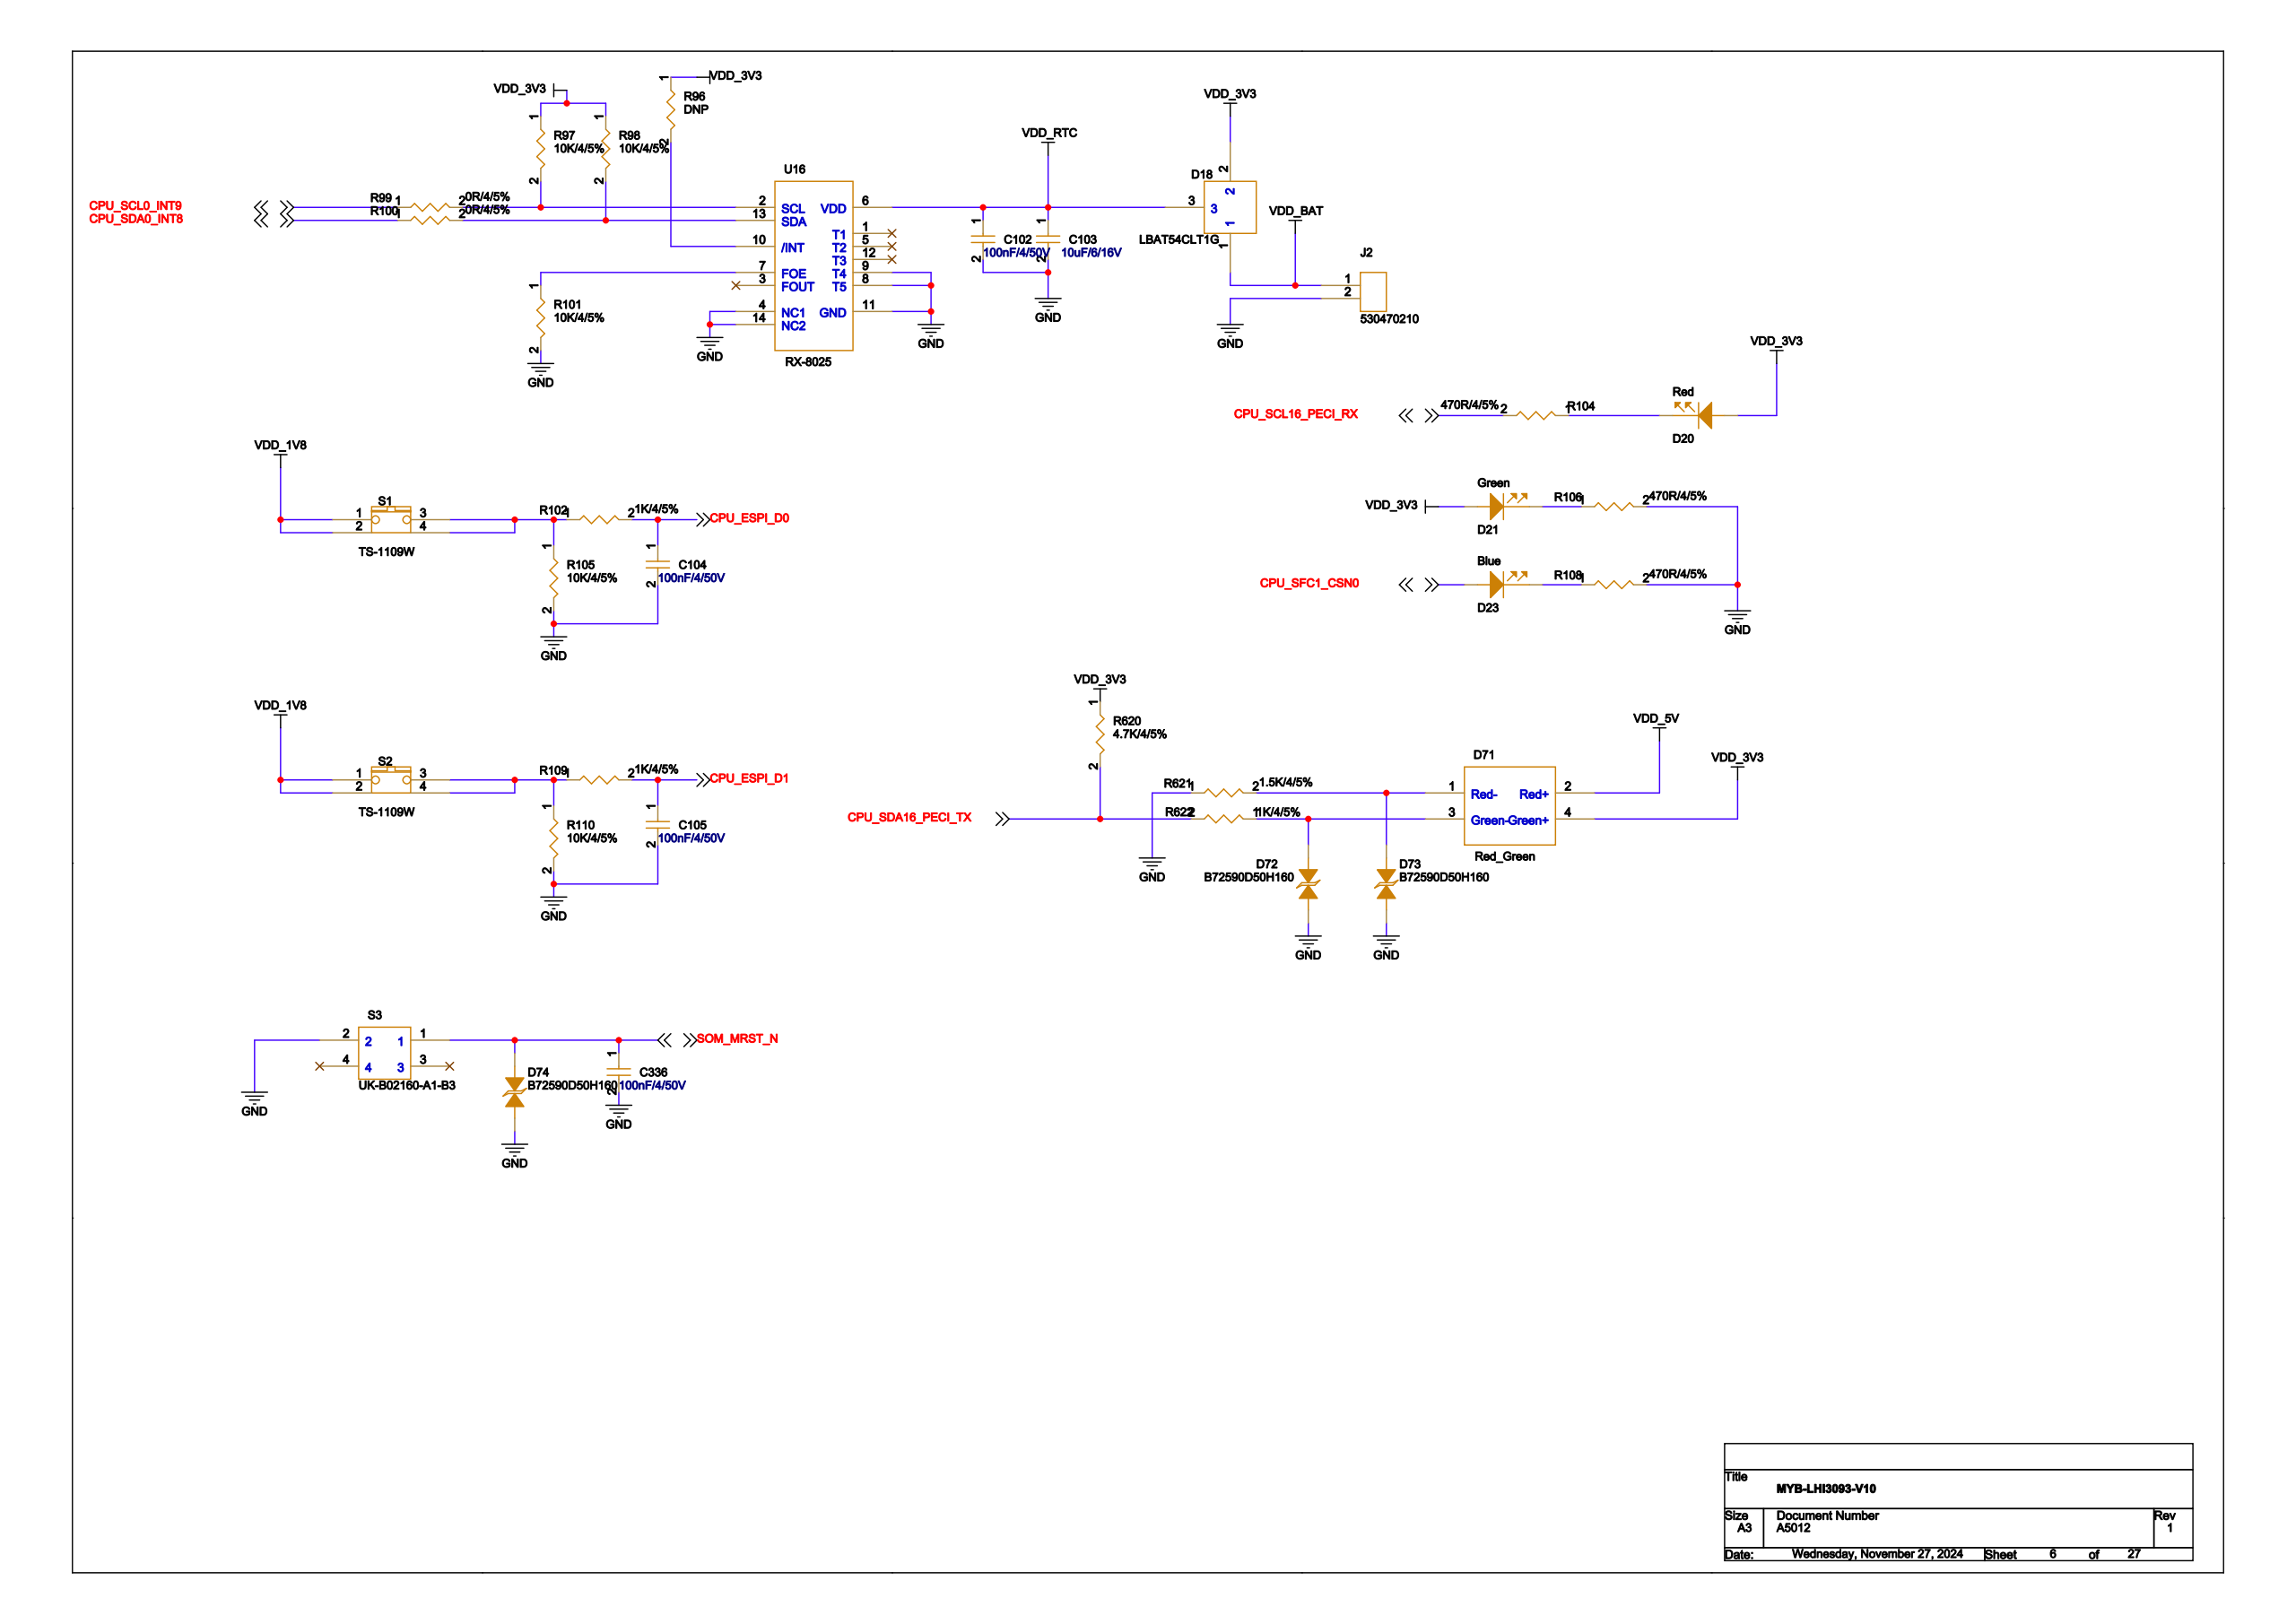Circuit board | Cadence Allegro | 1159 parts | 708 nets | one sheet of the schematic
Parts on this sheet (reference | value | footprint):
C102 | 100nF/4/50V | C0402
C103 | 10uF/6/16V | C0603
C104 | 100nF/4/50V | C0402
C105 | 100nF/4/50V | C0402
C336 | 100nF/4/50V | C0402
D18 | LBAT54CLT1G | SOT-23
D20 | LED-SML1206 | LED0603
D21 | LED-SML1206 | LED0603
D71 | Red_Green | LEDP-A694B
D72 | B72590D50H160 | D0402
D73 | B72590D50H160 | D0402
D74 | B72590D50H160 | D0402
J2 | 530470210 | CONN1X2-1_25-DIP
R96 | DNP | R0402
R97 | 10K/4/5% | R0402
R98 | 10K/4/5% | R0402
R99 | 0R/4/5% | R0402
R101 | 10K/4/5% | R0402
R105 | 10K/4/5% | R0402
R110 | 10K/4/5% | R0402
R620 | 4.7K/4/5% | R0402
S1 | TS-1109W | KEY-TS-1109W
S2 | TS-1109W | KEY-TS-1109W
S3 | UK-B02160-A1-B3 | UK-B02160-A1-B3
U16 | RX-8025 | SOP14
Nets of these parts (net: part-pin ...):
GND: C102-2 C103-2 C104-2 C105-2 C336-2 D72-1 D73-1 D74-1 J2-2 R101-2 R105-2 R110-2 S3-2 U16-4 U16-8 U16-9 U16-11 U16-14
VDD_5V: D71-2
VDD_RTC: C102-1 C103-1 D18-3 U16-6
CPU_ESPI_D0: C104-1
CPU_ESPI_D1: C105-1
VDD_3V3: D18-2 D20-1 D21-1 D71-4 R96-1 R97-1 R98-1 R620-1
VDD_1V8: S1-1 S1-2 S2-1 S2-2
SOM_MRST_N: C336-1 D74-2 S3-1
VDD_BAT: D18-1 J2-1
N14951283: D20-2
N14952859: D21-2
N14953430: D71-3 D72-2
N14953426: D71-1 D73-2
CPU_SCL0_INT9: R99-1
N14949975: R98-2 U16-13
N14949971: R97-2 R99-2 U16-2
N14950270: R101-1 U16-7
N14951410: R105-1 S1-3 S1-4
N14951894: R110-1 S2-3 S2-4
CPU_SDA16_PECI_TX: R620-2
N14950144: R96-2 U16-10